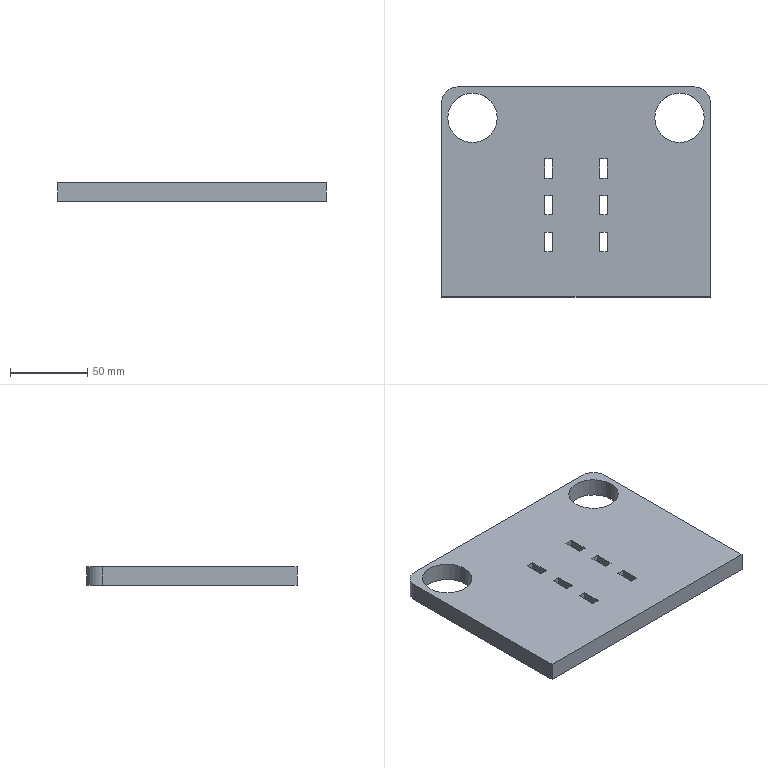Part | SolidWorks | features Extrusion 1, Fillet 1 | 1 solid | 36 faces | box 174 x 136 x 12 mm | volume 259651 mm3 | plane 30 | cylinder 6 | commonest cylinder face diameters 32 x4 20 x2
STEP:
#1=CARTESIAN_POINT('',(28.335,49.66,12.));
#2=VERTEX_POINT('',#1);
#3=CARTESIAN_POINT('',(60.335,49.66,12.));
#4=VERTEX_POINT('',#3);
#5=CARTESIAN_POINT('',(44.335,49.66,12.));
#6=DIRECTION('',(0.,0.,1.));
#7=DIRECTION('',(-1.,0.,0.));
#8=AXIS2_PLACEMENT_3D('',#5,#6,#7);
#9=CIRCLE('',#8,16.);
#10=EDGE_CURVE('',#2,#4,#9,.T.);
#11=ORIENTED_EDGE('',*,*,#10,.T.);
#12=CARTESIAN_POINT('',(60.335,49.66,0.));
#13=VERTEX_POINT('',#12);
#14=CARTESIAN_POINT('',(60.335,49.66,12.));
#15=DIRECTION('',(0.,0.,-1.));
#16=VECTOR('',#15,1000.);
#17=LINE('',#14,#16);
#18=EDGE_CURVE('',#4,#13,#17,.T.);
#19=ORIENTED_EDGE('',*,*,#18,.T.);
#20=CARTESIAN_POINT('',(28.335,49.66,0.));
#21=VERTEX_POINT('',#20);
#22=CARTESIAN_POINT('',(44.335,49.66,0.));
#23=DIRECTION('',(0.,0.,1.));
#24=DIRECTION('',(-1.,0.,0.));
#25=AXIS2_PLACEMENT_3D('',#22,#23,#24);
#26=CIRCLE('',#25,16.);
#27=EDGE_CURVE('',#21,#13,#26,.T.);
#28=ORIENTED_EDGE('',*,*,#27,.F.);
#29=CARTESIAN_POINT('',(28.335,49.66,12.));
#30=DIRECTION('',(0.,0.,-1.));
#31=VECTOR('',#30,1000.);
#32=LINE('',#29,#31);
#33=EDGE_CURVE('',#2,#21,#32,.T.);
#34=ORIENTED_EDGE('',*,*,#33,.F.);
#35=EDGE_LOOP('',(#11,#19,#28,#34));
#36=FACE_OUTER_BOUND('',#35,.T.);
#37=CARTESIAN_POINT('',(44.335,49.66,12.));
#38=DIRECTION('',(0.,0.,-1.));
#39=DIRECTION('',(-1.,0.,0.));
#40=AXIS2_PLACEMENT_3D('',#37,#38,#39);
#41=CYLINDRICAL_SURFACE('',#40,16.);
#42=ADVANCED_FACE('',(#36),#41,.F.);
#43=CARTESIAN_POINT('',(-105.665,49.66,12.));
#44=VERTEX_POINT('',#43);
#45=CARTESIAN_POINT('',(-73.665,49.66,12.));
#46=VERTEX_POINT('',#45);
#47=CARTESIAN_POINT('',(-89.665,49.66,12.));
#48=DIRECTION('',(0.,0.,1.));
#49=DIRECTION('',(1.,0.,0.));
#50=AXIS2_PLACEMENT_3D('',#47,#48,#49);
#51=CIRCLE('',#50,16.);
#52=EDGE_CURVE('',#44,#46,#51,.T.);
#53=ORIENTED_EDGE('',*,*,#52,.T.);
#54=CARTESIAN_POINT('',(-73.665,49.66,0.));
#55=VERTEX_POINT('',#54);
#56=CARTESIAN_POINT('',(-73.665,49.66,12.));
#57=DIRECTION('',(0.,0.,-1.));
#58=VECTOR('',#57,1000.);
#59=LINE('',#56,#58);
#60=EDGE_CURVE('',#46,#55,#59,.T.);
#61=ORIENTED_EDGE('',*,*,#60,.T.);
#62=CARTESIAN_POINT('',(-105.665,49.66,0.));
#63=VERTEX_POINT('',#62);
#64=CARTESIAN_POINT('',(-89.665,49.66,0.));
#65=DIRECTION('',(0.,0.,1.));
#66=DIRECTION('',(1.,0.,0.));
#67=AXIS2_PLACEMENT_3D('',#64,#65,#66);
#68=CIRCLE('',#67,16.);
#69=EDGE_CURVE('',#63,#55,#68,.T.);
#70=ORIENTED_EDGE('',*,*,#69,.F.);
#71=CARTESIAN_POINT('',(-105.665,49.66,12.));
#72=DIRECTION('',(0.,0.,-1.));
#73=VECTOR('',#72,1000.);
#74=LINE('',#71,#73);
#75=EDGE_CURVE('',#44,#63,#74,.T.);
#76=ORIENTED_EDGE('',*,*,#75,.F.);
#77=EDGE_LOOP('',(#53,#61,#70,#76));
#78=FACE_OUTER_BOUND('',#77,.T.);
#79=CARTESIAN_POINT('',(-89.665,49.66,12.));
#80=DIRECTION('',(0.,0.,-1.));
#81=DIRECTION('',(-1.,0.,0.));
#82=AXIS2_PLACEMENT_3D('',#79,#80,#81);
#83=CYLINDRICAL_SURFACE('',#82,16.);
#84=ADVANCED_FACE('',(#78),#83,.F.);
#85=CARTESIAN_POINT('',(-7.415,-0.6475,12.));
#86=VERTEX_POINT('',#85);
#87=CARTESIAN_POINT('',(-7.415,-13.148,12.));
#88=VERTEX_POINT('',#87);
#89=CARTESIAN_POINT('',(-7.415,-0.6475,12.));
#90=DIRECTION('',(0.,-1.,0.));
#91=VECTOR('',#90,1000.);
#92=LINE('',#89,#91);
#93=EDGE_CURVE('',#86,#88,#92,.T.);
#94=ORIENTED_EDGE('',*,*,#93,.F.);
#95=CARTESIAN_POINT('',(-2.415,-0.6475,12.));
#96=VERTEX_POINT('',#95);
#97=CARTESIAN_POINT('',(-7.415,-0.6475,12.));
#98=DIRECTION('',(-1.,0.,0.));
#99=VECTOR('',#98,1000.);
#100=LINE('',#97,#99);
#101=EDGE_CURVE('',#96,#86,#100,.T.);
#102=ORIENTED_EDGE('',*,*,#101,.F.);
#103=CARTESIAN_POINT('',(-2.415,-13.148,12.));
#104=VERTEX_POINT('',#103);
#105=CARTESIAN_POINT('',(-2.415,-0.6475,12.));
#106=DIRECTION('',(0.,1.,0.));
#107=VECTOR('',#106,1000.);
#108=LINE('',#105,#107);
#109=EDGE_CURVE('',#104,#96,#108,.T.);
#110=ORIENTED_EDGE('',*,*,#109,.F.);
#111=CARTESIAN_POINT('',(-2.415,-13.148,12.));
#112=DIRECTION('',(1.,0.,0.));
#113=VECTOR('',#112,1000.);
#114=LINE('',#111,#113);
#115=EDGE_CURVE('',#88,#104,#114,.T.);
#116=ORIENTED_EDGE('',*,*,#115,.F.);
#117=EDGE_LOOP('',(#94,#102,#110,#116));
#118=FACE_BOUND('',#117,.T.);
#119=CARTESIAN_POINT('',(-37.915,-36.898,12.));
#120=VERTEX_POINT('',#119);
#121=CARTESIAN_POINT('',(-37.915,-24.398,12.));
#122=VERTEX_POINT('',#121);
#123=CARTESIAN_POINT('',(-37.915,-24.398,12.));
#124=DIRECTION('',(0.,1.,0.));
#125=VECTOR('',#124,1000.);
#126=LINE('',#123,#125);
#127=EDGE_CURVE('',#120,#122,#126,.T.);
#128=ORIENTED_EDGE('',*,*,#127,.F.);
#129=CARTESIAN_POINT('',(-42.915,-36.898,12.));
#130=VERTEX_POINT('',#129);
#131=CARTESIAN_POINT('',(-42.915,-36.898,12.));
#132=DIRECTION('',(1.,0.,0.));
#133=VECTOR('',#132,1000.);
#134=LINE('',#131,#133);
#135=EDGE_CURVE('',#130,#120,#134,.T.);
#136=ORIENTED_EDGE('',*,*,#135,.F.);
#137=CARTESIAN_POINT('',(-42.915,-24.398,12.));
#138=VERTEX_POINT('',#137);
#139=CARTESIAN_POINT('',(-42.915,-24.398,12.));
#140=DIRECTION('',(0.,-1.,0.));
#141=VECTOR('',#140,1000.);
#142=LINE('',#139,#141);
#143=EDGE_CURVE('',#138,#130,#142,.T.);
#144=ORIENTED_EDGE('',*,*,#143,.F.);
#145=CARTESIAN_POINT('',(-37.915,-24.398,12.));
#146=DIRECTION('',(-1.,0.,0.));
#147=VECTOR('',#146,1000.);
#148=LINE('',#145,#147);
#149=EDGE_CURVE('',#122,#138,#148,.T.);
#150=ORIENTED_EDGE('',*,*,#149,.F.);
#151=EDGE_LOOP('',(#128,#136,#144,#150));
#152=FACE_BOUND('',#151,.T.);
#153=CARTESIAN_POINT('',(-37.915,10.602,12.));
#154=VERTEX_POINT('',#153);
#155=CARTESIAN_POINT('',(-37.915,23.102,12.));
#156=VERTEX_POINT('',#155);
#157=CARTESIAN_POINT('',(-37.915,23.102,12.));
#158=DIRECTION('',(0.,1.,0.));
#159=VECTOR('',#158,1000.);
#160=LINE('',#157,#159);
#161=EDGE_CURVE('',#154,#156,#160,.T.);
#162=ORIENTED_EDGE('',*,*,#161,.F.);
#163=CARTESIAN_POINT('',(-42.915,10.602,12.));
#164=VERTEX_POINT('',#163);
#165=CARTESIAN_POINT('',(-42.915,10.602,12.));
#166=DIRECTION('',(1.,0.,0.));
#167=VECTOR('',#166,1000.);
#168=LINE('',#165,#167);
#169=EDGE_CURVE('',#164,#154,#168,.T.);
#170=ORIENTED_EDGE('',*,*,#169,.F.);
#171=CARTESIAN_POINT('',(-42.915,23.102,12.));
#172=VERTEX_POINT('',#171);
#173=CARTESIAN_POINT('',(-42.915,23.102,12.));
#174=DIRECTION('',(0.,-1.,0.));
#175=VECTOR('',#174,1000.);
#176=LINE('',#173,#175);
#177=EDGE_CURVE('',#172,#164,#176,.T.);
#178=ORIENTED_EDGE('',*,*,#177,.F.);
#179=CARTESIAN_POINT('',(-37.915,23.102,12.));
#180=DIRECTION('',(-1.,0.,0.));
#181=VECTOR('',#180,1000.);
#182=LINE('',#179,#181);
#183=EDGE_CURVE('',#156,#172,#182,.T.);
#184=ORIENTED_EDGE('',*,*,#183,.F.);
#185=EDGE_LOOP('',(#162,#170,#178,#184));
#186=FACE_BOUND('',#185,.T.);
#187=CARTESIAN_POINT('',(64.335,-66.34,12.));
#188=VERTEX_POINT('',#187);
#189=CARTESIAN_POINT('',(64.335,59.66,12.));
#190=VERTEX_POINT('',#189);
#191=CARTESIAN_POINT('',(64.335,69.66,12.));
#192=DIRECTION('',(0.,1.,0.));
#193=VECTOR('',#192,1000.);
#194=LINE('',#191,#193);
#195=EDGE_CURVE('',#188,#190,#194,.T.);
#196=ORIENTED_EDGE('',*,*,#195,.T.);
#197=CARTESIAN_POINT('',(54.335,69.66,12.));
#198=VERTEX_POINT('',#197);
#199=CARTESIAN_POINT('',(54.335,59.66,12.));
#200=DIRECTION('',(0.,0.,1.));
#201=DIRECTION('',(-1.,0.,0.));
#202=AXIS2_PLACEMENT_3D('',#199,#200,#201);
#203=CIRCLE('',#202,10.);
#204=EDGE_CURVE('',#190,#198,#203,.T.);
#205=ORIENTED_EDGE('',*,*,#204,.T.);
#206=CARTESIAN_POINT('',(-99.665,69.66,12.));
#207=VERTEX_POINT('',#206);
#208=CARTESIAN_POINT('',(-109.665,69.66,12.));
#209=DIRECTION('',(-1.,0.,0.));
#210=VECTOR('',#209,1000.);
#211=LINE('',#208,#210);
#212=EDGE_CURVE('',#198,#207,#211,.T.);
#213=ORIENTED_EDGE('',*,*,#212,.T.);
#214=CARTESIAN_POINT('',(-109.665,59.66,12.));
#215=VERTEX_POINT('',#214);
#216=CARTESIAN_POINT('',(-99.665,59.66,12.));
#217=DIRECTION('',(0.,0.,1.));
#218=DIRECTION('',(-1.,0.,0.));
#219=AXIS2_PLACEMENT_3D('',#216,#217,#218);
#220=CIRCLE('',#219,10.);
#221=EDGE_CURVE('',#207,#215,#220,.T.);
#222=ORIENTED_EDGE('',*,*,#221,.T.);
#223=CARTESIAN_POINT('',(-109.665,-66.34,12.));
#224=VERTEX_POINT('',#223);
#225=CARTESIAN_POINT('',(-109.665,69.66,12.));
#226=DIRECTION('',(0.,-1.,0.));
#227=VECTOR('',#226,1000.);
#228=LINE('',#225,#227);
#229=EDGE_CURVE('',#215,#224,#228,.T.);
#230=ORIENTED_EDGE('',*,*,#229,.T.);
#231=CARTESIAN_POINT('',(-109.665,-66.34,12.));
#232=DIRECTION('',(1.,0.,0.));
#233=VECTOR('',#232,1000.);
#234=LINE('',#231,#233);
#235=EDGE_CURVE('',#224,#188,#234,.T.);
#236=ORIENTED_EDGE('',*,*,#235,.T.);
#237=EDGE_LOOP('',(#196,#205,#213,#222,#230,#236));
#238=FACE_OUTER_BOUND('',#237,.T.);
#239=ORIENTED_EDGE('',*,*,#52,.F.);
#240=CARTESIAN_POINT('',(-89.665,49.66,12.));
#241=DIRECTION('',(0.,0.,1.));
#242=DIRECTION('',(1.,0.,0.));
#243=AXIS2_PLACEMENT_3D('',#240,#241,#242);
#244=CIRCLE('',#243,16.);
#245=EDGE_CURVE('',#46,#44,#244,.T.);
#246=ORIENTED_EDGE('',*,*,#245,.F.);
#247=EDGE_LOOP('',(#239,#246));
#248=FACE_BOUND('',#247,.T.);
#249=ORIENTED_EDGE('',*,*,#10,.F.);
#250=CARTESIAN_POINT('',(44.335,49.66,12.));
#251=DIRECTION('',(0.,0.,1.));
#252=DIRECTION('',(-1.,0.,0.));
#253=AXIS2_PLACEMENT_3D('',#250,#251,#252);
#254=CIRCLE('',#253,16.);
#255=EDGE_CURVE('',#4,#2,#254,.T.);
#256=ORIENTED_EDGE('',*,*,#255,.F.);
#257=EDGE_LOOP('',(#249,#256));
#258=FACE_BOUND('',#257,.T.);
#259=CARTESIAN_POINT('',(-37.915,-13.148,12.));
#260=VERTEX_POINT('',#259);
#261=CARTESIAN_POINT('',(-37.915,-0.6475,12.));
#262=VERTEX_POINT('',#261);
#263=CARTESIAN_POINT('',(-37.915,-0.6475,12.));
#264=DIRECTION('',(0.,1.,0.));
#265=VECTOR('',#264,1000.);
#266=LINE('',#263,#265);
#267=EDGE_CURVE('',#260,#262,#266,.T.);
#268=ORIENTED_EDGE('',*,*,#267,.F.);
#269=CARTESIAN_POINT('',(-42.915,-13.148,12.));
#270=VERTEX_POINT('',#269);
#271=CARTESIAN_POINT('',(-42.915,-13.148,12.));
#272=DIRECTION('',(1.,0.,0.));
#273=VECTOR('',#272,1000.);
#274=LINE('',#271,#273);
#275=EDGE_CURVE('',#270,#260,#274,.T.);
#276=ORIENTED_EDGE('',*,*,#275,.F.);
#277=CARTESIAN_POINT('',(-42.915,-0.6475,12.));
#278=VERTEX_POINT('',#277);
#279=CARTESIAN_POINT('',(-42.915,-0.6475,12.));
#280=DIRECTION('',(0.,-1.,0.));
#281=VECTOR('',#280,1000.);
#282=LINE('',#279,#281);
#283=EDGE_CURVE('',#278,#270,#282,.T.);
#284=ORIENTED_EDGE('',*,*,#283,.F.);
#285=CARTESIAN_POINT('',(-37.915,-0.6475,12.));
#286=DIRECTION('',(-1.,0.,0.));
#287=VECTOR('',#286,1000.);
#288=LINE('',#285,#287);
#289=EDGE_CURVE('',#262,#278,#288,.T.);
#290=ORIENTED_EDGE('',*,*,#289,.F.);
#291=EDGE_LOOP('',(#268,#276,#284,#290));
#292=FACE_BOUND('',#291,.T.);
#293=CARTESIAN_POINT('',(-7.415,-24.398,12.));
#294=VERTEX_POINT('',#293);
#295=CARTESIAN_POINT('',(-7.415,-36.898,12.));
#296=VERTEX_POINT('',#295);
#297=CARTESIAN_POINT('',(-7.415,-24.398,12.));
#298=DIRECTION('',(0.,-1.,0.));
#299=VECTOR('',#298,1000.);
#300=LINE('',#297,#299);
#301=EDGE_CURVE('',#294,#296,#300,.T.);
#302=ORIENTED_EDGE('',*,*,#301,.F.);
#303=CARTESIAN_POINT('',(-2.415,-24.398,12.));
#304=VERTEX_POINT('',#303);
#305=CARTESIAN_POINT('',(-7.415,-24.398,12.));
#306=DIRECTION('',(-1.,0.,0.));
#307=VECTOR('',#306,1000.);
#308=LINE('',#305,#307);
#309=EDGE_CURVE('',#304,#294,#308,.T.);
#310=ORIENTED_EDGE('',*,*,#309,.F.);
#311=CARTESIAN_POINT('',(-2.415,-36.898,12.));
#312=VERTEX_POINT('',#311);
#313=CARTESIAN_POINT('',(-2.415,-24.398,12.));
#314=DIRECTION('',(0.,1.,0.));
#315=VECTOR('',#314,1000.);
#316=LINE('',#313,#315);
#317=EDGE_CURVE('',#312,#304,#316,.T.);
#318=ORIENTED_EDGE('',*,*,#317,.F.);
#319=CARTESIAN_POINT('',(-2.415,-36.898,12.));
#320=DIRECTION('',(1.,0.,0.));
#321=VECTOR('',#320,1000.);
#322=LINE('',#319,#321);
#323=EDGE_CURVE('',#296,#312,#322,.T.);
#324=ORIENTED_EDGE('',*,*,#323,.F.);
#325=EDGE_LOOP('',(#302,#310,#318,#324));
#326=FACE_BOUND('',#325,.T.);
#327=CARTESIAN_POINT('',(-7.415,23.102,12.));
#328=VERTEX_POINT('',#327);
#329=CARTESIAN_POINT('',(-7.415,10.602,12.));
#330=VERTEX_POINT('',#329);
#331=CARTESIAN_POINT('',(-7.415,23.102,12.));
#332=DIRECTION('',(0.,-1.,0.));
#333=VECTOR('',#332,1000.);
#334=LINE('',#331,#333);
#335=EDGE_CURVE('',#328,#330,#334,.T.);
#336=ORIENTED_EDGE('',*,*,#335,.F.);
#337=CARTESIAN_POINT('',(-2.415,23.102,12.));
#338=VERTEX_POINT('',#337);
#339=CARTESIAN_POINT('',(-7.415,23.102,12.));
#340=DIRECTION('',(-1.,0.,0.));
#341=VECTOR('',#340,1000.);
#342=LINE('',#339,#341);
#343=EDGE_CURVE('',#338,#328,#342,.T.);
#344=ORIENTED_EDGE('',*,*,#343,.F.);
#345=CARTESIAN_POINT('',(-2.415,10.602,12.));
#346=VERTEX_POINT('',#345);
#347=CARTESIAN_POINT('',(-2.415,23.102,12.));
#348=DIRECTION('',(0.,1.,0.));
#349=VECTOR('',#348,1000.);
#350=LINE('',#347,#349);
#351=EDGE_CURVE('',#346,#338,#350,.T.);
#352=ORIENTED_EDGE('',*,*,#351,.F.);
#353=CARTESIAN_POINT('',(-2.415,10.602,12.));
#354=DIRECTION('',(1.,0.,0.));
#355=VECTOR('',#354,1000.);
#356=LINE('',#353,#355);
#357=EDGE_CURVE('',#330,#346,#356,.T.);
#358=ORIENTED_EDGE('',*,*,#357,.F.);
#359=EDGE_LOOP('',(#336,#344,#352,#358));
#360=FACE_BOUND('',#359,.T.);
#361=CARTESIAN_POINT('',(0.,0.,12.));
#362=DIRECTION('',(0.,0.,-1.));
#363=DIRECTION('',(-1.,0.,0.));
#364=AXIS2_PLACEMENT_3D('',#361,#362,#363);
#365=PLANE('',#364);
#366=ADVANCED_FACE('',(#118,#152,#186,#238,#248,#258,#292,#326,#360),#365,.F.);
#367=ORIENTED_EDGE('',*,*,#69,.T.);
#368=CARTESIAN_POINT('',(-89.665,49.66,0.));
#369=DIRECTION('',(0.,0.,1.));
#370=DIRECTION('',(1.,0.,0.));
#371=AXIS2_PLACEMENT_3D('',#368,#369,#370);
#372=CIRCLE('',#371,16.);
#373=EDGE_CURVE('',#55,#63,#372,.T.);
#374=ORIENTED_EDGE('',*,*,#373,.T.);
#375=EDGE_LOOP('',(#367,#374));
#376=FACE_BOUND('',#375,.T.);
#377=CARTESIAN_POINT('',(54.335,69.66,0.));
#378=VERTEX_POINT('',#377);
#379=CARTESIAN_POINT('',(-99.665,69.66,0.));
#380=VERTEX_POINT('',#379);
#381=CARTESIAN_POINT('',(-109.665,69.66,0.));
#382=DIRECTION('',(-1.,0.,0.));
#383=VECTOR('',#382,1000.);
#384=LINE('',#381,#383);
#385=EDGE_CURVE('',#378,#380,#384,.T.);
#386=ORIENTED_EDGE('',*,*,#385,.F.);
#387=CARTESIAN_POINT('',(64.335,59.66,0.));
#388=VERTEX_POINT('',#387);
#389=CARTESIAN_POINT('',(54.335,59.66,0.));
#390=DIRECTION('',(0.,0.,-1.));
#391=DIRECTION('',(-1.,0.,0.));
#392=AXIS2_PLACEMENT_3D('',#389,#390,#391);
#393=CIRCLE('',#392,10.);
#394=EDGE_CURVE('',#378,#388,#393,.T.);
#395=ORIENTED_EDGE('',*,*,#394,.T.);
#396=CARTESIAN_POINT('',(64.335,-66.34,0.));
#397=VERTEX_POINT('',#396);
#398=CARTESIAN_POINT('',(64.335,69.66,0.));
#399=DIRECTION('',(0.,1.,0.));
#400=VECTOR('',#399,1000.);
#401=LINE('',#398,#400);
#402=EDGE_CURVE('',#397,#388,#401,.T.);
#403=ORIENTED_EDGE('',*,*,#402,.F.);
#404=CARTESIAN_POINT('',(-109.665,-66.34,0.));
#405=VERTEX_POINT('',#404);
#406=CARTESIAN_POINT('',(-109.665,-66.34,0.));
#407=DIRECTION('',(1.,0.,0.));
#408=VECTOR('',#407,1000.);
#409=LINE('',#406,#408);
#410=EDGE_CURVE('',#405,#397,#409,.T.);
#411=ORIENTED_EDGE('',*,*,#410,.F.);
#412=CARTESIAN_POINT('',(-109.665,59.66,0.));
#413=VERTEX_POINT('',#412);
#414=CARTESIAN_POINT('',(-109.665,69.66,0.));
#415=DIRECTION('',(0.,-1.,0.));
#416=VECTOR('',#415,1000.);
#417=LINE('',#414,#416);
#418=EDGE_CURVE('',#413,#405,#417,.T.);
#419=ORIENTED_EDGE('',*,*,#418,.F.);
#420=CARTESIAN_POINT('',(-99.665,59.66,0.));
#421=DIRECTION('',(0.,0.,-1.));
#422=DIRECTION('',(-1.,0.,0.));
#423=AXIS2_PLACEMENT_3D('',#420,#421,#422);
#424=CIRCLE('',#423,10.);
#425=EDGE_CURVE('',#413,#380,#424,.T.);
#426=ORIENTED_EDGE('',*,*,#425,.T.);
#427=EDGE_LOOP('',(#386,#395,#403,#411,#419,#426));
#428=FACE_OUTER_BOUND('',#427,.T.);
#429=ORIENTED_EDGE('',*,*,#27,.T.);
#430=CARTESIAN_POINT('',(44.335,49.66,0.));
#431=DIRECTION('',(0.,0.,1.));
#432=DIRECTION('',(-1.,0.,0.));
#433=AXIS2_PLACEMENT_3D('',#430,#431,#432);
#434=CIRCLE('',#433,16.);
#435=EDGE_CURVE('',#13,#21,#434,.T.);
#436=ORIENTED_EDGE('',*,*,#435,.T.);
#437=EDGE_LOOP('',(#429,#436));
#438=FACE_BOUND('',#437,.T.);
#439=CARTESIAN_POINT('',(-42.915,10.602,0.));
#440=VERTEX_POINT('',#439);
#441=CARTESIAN_POINT('',(-37.915,10.602,0.));
#442=VERTEX_POINT('',#441);
#443=CARTESIAN_POINT('',(-42.915,10.602,0.));
#444=DIRECTION('',(1.,0.,0.));
#445=VECTOR('',#444,1000.);
#446=LINE('',#443,#445);
#447=EDGE_CURVE('',#440,#442,#446,.T.);
#448=ORIENTED_EDGE('',*,*,#447,.T.);
#449=CARTESIAN_POINT('',(-37.915,23.102,0.));
#450=VERTEX_POINT('',#449);
#451=CARTESIAN_POINT('',(-37.915,23.102,0.));
#452=DIRECTION('',(0.,1.,0.));
#453=VECTOR('',#452,1000.);
#454=LINE('',#451,#453);
#455=EDGE_CURVE('',#442,#450,#454,.T.);
#456=ORIENTED_EDGE('',*,*,#455,.T.);
#457=CARTESIAN_POINT('',(-42.915,23.102,0.));
#458=VERTEX_POINT('',#457);
#459=CARTESIAN_POINT('',(-37.915,23.102,0.));
#460=DIRECTION('',(-1.,0.,0.));
#461=VECTOR('',#460,1000.);
#462=LINE('',#459,#461);
#463=EDGE_CURVE('',#450,#458,#462,.T.);
#464=ORIENTED_EDGE('',*,*,#463,.T.);
#465=CARTESIAN_POINT('',(-42.915,23.102,0.));
#466=DIRECTION('',(0.,-1.,0.));
#467=VECTOR('',#466,1000.);
#468=LINE('',#465,#467);
#469=EDGE_CURVE('',#458,#440,#468,.T.);
#470=ORIENTED_EDGE('',*,*,#469,.T.);
#471=EDGE_LOOP('',(#448,#456,#464,#470));
#472=FACE_BOUND('',#471,.T.);
#473=CARTESIAN_POINT('',(-42.915,-13.148,0.));
#474=VERTEX_POINT('',#473);
#475=CARTESIAN_POINT('',(-37.915,-13.148,0.));
#476=VERTEX_POINT('',#475);
#477=CARTESIAN_POINT('',(-42.915,-13.148,0.));
#478=DIRECTION('',(1.,0.,0.));
#479=VECTOR('',#478,1000.);
#480=LINE('',#477,#479);
#481=EDGE_CURVE('',#474,#476,#480,.T.);
#482=ORIENTED_EDGE('',*,*,#481,.T.);
#483=CARTESIAN_POINT('',(-37.915,-0.6475,0.));
#484=VERTEX_POINT('',#483);
#485=CARTESIAN_POINT('',(-37.915,-0.6475,0.));
#486=DIRECTION('',(0.,1.,0.));
#487=VECTOR('',#486,1000.);
#488=LINE('',#485,#487);
#489=EDGE_CURVE('',#476,#484,#488,.T.);
#490=ORIENTED_EDGE('',*,*,#489,.T.);
#491=CARTESIAN_POINT('',(-42.915,-0.6475,0.));
#492=VERTEX_POINT('',#491);
#493=CARTESIAN_POINT('',(-37.915,-0.6475,0.));
#494=DIRECTION('',(-1.,0.,0.));
#495=VECTOR('',#494,1000.);
#496=LINE('',#493,#495);
#497=EDGE_CURVE('',#484,#492,#496,.T.);
#498=ORIENTED_EDGE('',*,*,#497,.T.);
#499=CARTESIAN_POINT('',(-42.915,-0.6475,0.));
#500=DIRECTION('',(0.,-1.,0.));
#501=VECTOR('',#500,1000.);
#502=LINE('',#499,#501);
#503=EDGE_CURVE('',#492,#474,#502,.T.);
#504=ORIENTED_EDGE('',*,*,#503,.T.);
#505=EDGE_LOOP('',(#482,#490,#498,#504));
#506=FACE_BOUND('',#505,.T.);
#507=CARTESIAN_POINT('',(-42.915,-36.898,0.));
#508=VERTEX_POINT('',#507);
#509=CARTESIAN_POINT('',(-37.915,-36.898,0.));
#510=VERTEX_POINT('',#509);
#511=CARTESIAN_POINT('',(-42.915,-36.898,0.));
#512=DIRECTION('',(1.,0.,0.));
#513=VECTOR('',#512,1000.);
#514=LINE('',#511,#513);
#515=EDGE_CURVE('',#508,#510,#514,.T.);
#516=ORIENTED_EDGE('',*,*,#515,.T.);
#517=CARTESIAN_POINT('',(-37.915,-24.398,0.));
#518=VERTEX_POINT('',#517);
#519=CARTESIAN_POINT('',(-37.915,-24.398,0.));
#520=DIRECTION('',(0.,1.,0.));
#521=VECTOR('',#520,1000.);
#522=LINE('',#519,#521);
#523=EDGE_CURVE('',#510,#518,#522,.T.);
#524=ORIENTED_EDGE('',*,*,#523,.T.);
#525=CARTESIAN_POINT('',(-42.915,-24.398,0.));
#526=VERTEX_POINT('',#525);
#527=CARTESIAN_POINT('',(-37.915,-24.398,0.));
#528=DIRECTION('',(-1.,0.,0.));
#529=VECTOR('',#528,1000.);
#530=LINE('',#527,#529);
#531=EDGE_CURVE('',#518,#526,#530,.T.);
#532=ORIENTED_EDGE('',*,*,#531,.T.);
#533=CARTESIAN_POINT('',(-42.915,-24.398,0.));
#534=DIRECTION('',(0.,-1.,0.));
#535=VECTOR('',#534,1000.);
#536=LINE('',#533,#535);
#537=EDGE_CURVE('',#526,#508,#536,.T.);
#538=ORIENTED_EDGE('',*,*,#537,.T.);
#539=EDGE_LOOP('',(#516,#524,#532,#538));
#540=FACE_BOUND('',#539,.T.);
#541=CARTESIAN_POINT('',(-2.415,-24.398,0.));
#542=VERTEX_POINT('',#541);
#543=CARTESIAN_POINT('',(-7.415,-24.398,0.));
#544=VERTEX_POINT('',#543);
#545=CARTESIAN_POINT('',(-7.415,-24.398,0.));
#546=DIRECTION('',(-1.,0.,0.));
#547=VECTOR('',#546,1000.);
#548=LINE('',#545,#547);
#549=EDGE_CURVE('',#542,#544,#548,.T.);
#550=ORIENTED_EDGE('',*,*,#549,.T.);
#551=CARTESIAN_POINT('',(-7.415,-36.898,0.));
#552=VERTEX_POINT('',#551);
#553=CARTESIAN_POINT('',(-7.415,-24.398,0.));
#554=DIRECTION('',(0.,-1.,0.));
#555=VECTOR('',#554,1000.);
#556=LINE('',#553,#555);
#557=EDGE_CURVE('',#544,#552,#556,.T.);
#558=ORIENTED_EDGE('',*,*,#557,.T.);
#559=CARTESIAN_POINT('',(-2.415,-36.898,0.));
#560=VERTEX_POINT('',#559);
#561=CARTESIAN_POINT('',(-2.415,-36.898,0.));
#562=DIRECTION('',(1.,0.,0.));
#563=VECTOR('',#562,1000.);
#564=LINE('',#561,#563);
#565=EDGE_CURVE('',#552,#560,#564,.T.);
#566=ORIENTED_EDGE('',*,*,#565,.T.);
#567=CARTESIAN_POINT('',(-2.415,-24.398,0.));
#568=DIRECTION('',(0.,1.,0.));
#569=VECTOR('',#568,1000.);
#570=LINE('',#567,#569);
#571=EDGE_CURVE('',#560,#542,#570,.T.);
#572=ORIENTED_EDGE('',*,*,#571,.T.);
#573=EDGE_LOOP('',(#550,#558,#566,#572));
#574=FACE_BOUND('',#573,.T.);
#575=CARTESIAN_POINT('',(-2.415,-0.6475,0.));
#576=VERTEX_POINT('',#575);
#577=CARTESIAN_POINT('',(-7.415,-0.6475,0.));
#578=VERTEX_POINT('',#577);
#579=CARTESIAN_POINT('',(-7.415,-0.6475,0.));
#580=DIRECTION('',(-1.,0.,0.));
#581=VECTOR('',#580,1000.);
#582=LINE('',#579,#581);
#583=EDGE_CURVE('',#576,#578,#582,.T.);
#584=ORIENTED_EDGE('',*,*,#583,.T.);
#585=CARTESIAN_POINT('',(-7.415,-13.148,0.));
#586=VERTEX_POINT('',#585);
#587=CARTESIAN_POINT('',(-7.415,-0.6475,0.));
#588=DIRECTION('',(0.,-1.,0.));
#589=VECTOR('',#588,1000.);
#590=LINE('',#587,#589);
#591=EDGE_CURVE('',#578,#586,#590,.T.);
#592=ORIENTED_EDGE('',*,*,#591,.T.);
#593=CARTESIAN_POINT('',(-2.415,-13.148,0.));
#594=VERTEX_POINT('',#593);
#595=CARTESIAN_POINT('',(-2.415,-13.148,0.));
#596=DIRECTION('',(1.,0.,0.));
#597=VECTOR('',#596,1000.);
#598=LINE('',#595,#597);
#599=EDGE_CURVE('',#586,#594,#598,.T.);
#600=ORIENTED_EDGE('',*,*,#599,.T.);
#601=CARTESIAN_POINT('',(-2.415,-0.6475,0.));
#602=DIRECTION('',(0.,1.,0.));
#603=VECTOR('',#602,1000.);
#604=LINE('',#601,#603);
#605=EDGE_CURVE('',#594,#576,#604,.T.);
#606=ORIENTED_EDGE('',*,*,#605,.T.);
#607=EDGE_LOOP('',(#584,#592,#600,#606));
#608=FACE_BOUND('',#607,.T.);
#609=CARTESIAN_POINT('',(-2.415,23.102,0.));
#610=VERTEX_POINT('',#609);
#611=CARTESIAN_POINT('',(-7.415,23.102,0.));
#612=VERTEX_POINT('',#611);
#613=CARTESIAN_POINT('',(-7.415,23.102,0.));
#614=DIRECTION('',(-1.,0.,0.));
#615=VECTOR('',#614,1000.);
#616=LINE('',#613,#615);
#617=EDGE_CURVE('',#610,#612,#616,.T.);
#618=ORIENTED_EDGE('',*,*,#617,.T.);
#619=CARTESIAN_POINT('',(-7.415,10.602,0.));
#620=VERTEX_POINT('',#619);
#621=CARTESIAN_POINT('',(-7.415,23.102,0.));
#622=DIRECTION('',(0.,-1.,0.));
#623=VECTOR('',#622,1000.);
#624=LINE('',#621,#623);
#625=EDGE_CURVE('',#612,#620,#624,.T.);
#626=ORIENTED_EDGE('',*,*,#625,.T.);
#627=CARTESIAN_POINT('',(-2.415,10.602,0.));
#628=VERTEX_POINT('',#627);
#629=CARTESIAN_POINT('',(-2.415,10.602,0.));
#630=DIRECTION('',(1.,0.,0.));
#631=VECTOR('',#630,1000.);
#632=LINE('',#629,#631);
#633=EDGE_CURVE('',#620,#628,#632,.T.);
#634=ORIENTED_EDGE('',*,*,#633,.T.);
#635=CARTESIAN_POINT('',(-2.415,23.102,0.));
#636=DIRECTION('',(0.,1.,0.));
#637=VECTOR('',#636,1000.);
#638=LINE('',#635,#637);
#639=EDGE_CURVE('',#628,#610,#638,.T.);
#640=ORIENTED_EDGE('',*,*,#639,.T.);
#641=EDGE_LOOP('',(#618,#626,#634,#640));
#642=FACE_BOUND('',#641,.T.);
#643=CARTESIAN_POINT('',(0.,0.,0.));
#644=DIRECTION('',(0.,0.,-1.));
#645=DIRECTION('',(-1.,0.,0.));
#646=AXIS2_PLACEMENT_3D('',#643,#644,#645);
#647=PLANE('',#646);
#648=ADVANCED_FACE('',(#376,#428,#438,#472,#506,#540,#574,#608,#642),#647,.T.);
#649=ORIENTED_EDGE('',*,*,#212,.F.);
#650=CARTESIAN_POINT('',(54.335,69.66,12.));
#651=DIRECTION('',(0.,0.,-1.));
#652=VECTOR('',#651,1000.);
#653=LINE('',#650,#652);
#654=EDGE_CURVE('',#198,#378,#653,.T.);
#655=ORIENTED_EDGE('',*,*,#654,.T.);
#656=ORIENTED_EDGE('',*,*,#385,.T.);
#657=CARTESIAN_POINT('',(-99.665,69.66,12.));
#658=DIRECTION('',(0.,0.,1.));
#659=VECTOR('',#658,1000.);
#660=LINE('',#657,#659);
#661=EDGE_CURVE('',#380,#207,#660,.T.);
#662=ORIENTED_EDGE('',*,*,#661,.T.);
#663=EDGE_LOOP('',(#649,#655,#656,#662));
#664=FACE_OUTER_BOUND('',#663,.T.);
#665=CARTESIAN_POINT('',(-109.665,69.66,12.));
#666=DIRECTION('',(0.,-1.,0.));
#667=DIRECTION('',(0.,0.,-1.));
#668=AXIS2_PLACEMENT_3D('',#665,#666,#667);
#669=PLANE('',#668);
#670=ADVANCED_FACE('',(#664),#669,.F.);
#671=ORIENTED_EDGE('',*,*,#229,.F.);
#672=CARTESIAN_POINT('',(-109.665,59.66,12.));
#673=DIRECTION('',(0.,0.,-1.));
#674=VECTOR('',#673,1000.);
#675=LINE('',#672,#674);
#676=EDGE_CURVE('',#215,#413,#675,.T.);
#677=ORIENTED_EDGE('',*,*,#676,.T.);
#678=ORIENTED_EDGE('',*,*,#418,.T.);
#679=CARTESIAN_POINT('',(-109.665,-66.34,12.));
#680=DIRECTION('',(0.,0.,-1.));
#681=VECTOR('',#680,1000.);
#682=LINE('',#679,#681);
#683=EDGE_CURVE('',#224,#405,#682,.T.);
#684=ORIENTED_EDGE('',*,*,#683,.F.);
#685=EDGE_LOOP('',(#671,#677,#678,#684));
#686=FACE_OUTER_BOUND('',#685,.T.);
#687=CARTESIAN_POINT('',(-109.665,69.66,12.));
#688=DIRECTION('',(1.,0.,0.));
#689=DIRECTION('',(0.,1.,0.));
#690=AXIS2_PLACEMENT_3D('',#687,#688,#689);
#691=PLANE('',#690);
#692=ADVANCED_FACE('',(#686),#691,.F.);
#693=ORIENTED_EDGE('',*,*,#410,.T.);
#694=CARTESIAN_POINT('',(64.335,-66.34,12.));
#695=DIRECTION('',(0.,0.,-1.));
#696=VECTOR('',#695,1000.);
#697=LINE('',#694,#696);
#698=EDGE_CURVE('',#188,#397,#697,.T.);
#699=ORIENTED_EDGE('',*,*,#698,.F.);
#700=ORIENTED_EDGE('',*,*,#235,.F.);
#701=ORIENTED_EDGE('',*,*,#683,.T.);
#702=EDGE_LOOP('',(#693,#699,#700,#701));
#703=FACE_OUTER_BOUND('',#702,.T.);
#704=CARTESIAN_POINT('',(-109.665,-66.34,12.));
#705=DIRECTION('',(0.,1.,0.));
#706=DIRECTION('',(0.,0.,1.));
#707=AXIS2_PLACEMENT_3D('',#704,#705,#706);
#708=PLANE('',#707);
#709=ADVANCED_FACE('',(#703),#708,.F.);
#710=ORIENTED_EDGE('',*,*,#402,.T.);
#711=CARTESIAN_POINT('',(64.335,59.66,12.));
#712=DIRECTION('',(0.,0.,1.));
#713=VECTOR('',#712,1000.);
#714=LINE('',#711,#713);
#715=EDGE_CURVE('',#388,#190,#714,.T.);
#716=ORIENTED_EDGE('',*,*,#715,.T.);
#717=ORIENTED_EDGE('',*,*,#195,.F.);
#718=ORIENTED_EDGE('',*,*,#698,.T.);
#719=EDGE_LOOP('',(#710,#716,#717,#718));
#720=FACE_OUTER_BOUND('',#719,.T.);
#721=CARTESIAN_POINT('',(64.335,69.66,12.));
#722=DIRECTION('',(-1.,0.,0.));
#723=DIRECTION('',(0.,-1.,0.));
#724=AXIS2_PLACEMENT_3D('',#721,#722,#723);
#725=PLANE('',#724);
#726=ADVANCED_FACE('',(#720),#725,.F.);
#727=ORIENTED_EDGE('',*,*,#60,.F.);
#728=ORIENTED_EDGE('',*,*,#245,.T.);
#729=ORIENTED_EDGE('',*,*,#75,.T.);
#730=ORIENTED_EDGE('',*,*,#373,.F.);
#731=EDGE_LOOP('',(#727,#728,#729,#730));
#732=FACE_OUTER_BOUND('',#731,.T.);
#733=CARTESIAN_POINT('',(-89.665,49.66,12.));
#734=DIRECTION('',(0.,0.,-1.));
#735=DIRECTION('',(-1.,0.,0.));
#736=AXIS2_PLACEMENT_3D('',#733,#734,#735);
#737=CYLINDRICAL_SURFACE('',#736,16.);
#738=ADVANCED_FACE('',(#732),#737,.F.);
#739=ORIENTED_EDGE('',*,*,#18,.F.);
#740=ORIENTED_EDGE('',*,*,#255,.T.);
#741=ORIENTED_EDGE('',*,*,#33,.T.);
#742=ORIENTED_EDGE('',*,*,#435,.F.);
#743=EDGE_LOOP('',(#739,#740,#741,#742));
#744=FACE_OUTER_BOUND('',#743,.T.);
#745=CARTESIAN_POINT('',(44.335,49.66,12.));
#746=DIRECTION('',(0.,0.,-1.));
#747=DIRECTION('',(-1.,0.,0.));
#748=AXIS2_PLACEMENT_3D('',#745,#746,#747);
#749=CYLINDRICAL_SURFACE('',#748,16.);
#750=ADVANCED_FACE('',(#744),#749,.F.);
#751=ORIENTED_EDGE('',*,*,#455,.F.);
#752=CARTESIAN_POINT('',(-37.915,10.602,12.));
#753=DIRECTION('',(0.,0.,-1.));
#754=VECTOR('',#753,1000.);
#755=LINE('',#752,#754);
#756=EDGE_CURVE('',#154,#442,#755,.T.);
#757=ORIENTED_EDGE('',*,*,#756,.F.);
#758=ORIENTED_EDGE('',*,*,#161,.T.);
#759=CARTESIAN_POINT('',(-37.915,23.102,12.));
#760=DIRECTION('',(0.,0.,-1.));
#761=VECTOR('',#760,1000.);
#762=LINE('',#759,#761);
#763=EDGE_CURVE('',#156,#450,#762,.T.);
#764=ORIENTED_EDGE('',*,*,#763,.T.);
#765=EDGE_LOOP('',(#751,#757,#758,#764));
#766=FACE_OUTER_BOUND('',#765,.T.);
#767=CARTESIAN_POINT('',(-37.915,23.102,12.));
#768=DIRECTION('',(-1.,0.,0.));
#769=DIRECTION('',(0.,0.,1.));
#770=AXIS2_PLACEMENT_3D('',#767,#768,#769);
#771=PLANE('',#770);
#772=ADVANCED_FACE('',(#766),#771,.T.);
#773=ORIENTED_EDGE('',*,*,#463,.F.);
#774=ORIENTED_EDGE('',*,*,#763,.F.);
#775=ORIENTED_EDGE('',*,*,#183,.T.);
#776=CARTESIAN_POINT('',(-42.915,23.102,12.));
#777=DIRECTION('',(0.,0.,-1.));
#778=VECTOR('',#777,1000.);
#779=LINE('',#776,#778);
#780=EDGE_CURVE('',#172,#458,#779,.T.);
#781=ORIENTED_EDGE('',*,*,#780,.T.);
#782=EDGE_LOOP('',(#773,#774,#775,#781));
#783=FACE_OUTER_BOUND('',#782,.T.);
#784=CARTESIAN_POINT('',(-37.915,23.102,12.));
#785=DIRECTION('',(0.,-1.,0.));
#786=DIRECTION('',(0.,0.,-1.));
#787=AXIS2_PLACEMENT_3D('',#784,#785,#786);
#788=PLANE('',#787);
#789=ADVANCED_FACE('',(#783),#788,.T.);
#790=ORIENTED_EDGE('',*,*,#469,.F.);
#791=ORIENTED_EDGE('',*,*,#780,.F.);
#792=ORIENTED_EDGE('',*,*,#177,.T.);
#793=CARTESIAN_POINT('',(-42.915,10.602,12.));
#794=DIRECTION('',(0.,0.,-1.));
#795=VECTOR('',#794,1000.);
#796=LINE('',#793,#795);
#797=EDGE_CURVE('',#164,#440,#796,.T.);
#798=ORIENTED_EDGE('',*,*,#797,.T.);
#799=EDGE_LOOP('',(#790,#791,#792,#798));
#800=FACE_OUTER_BOUND('',#799,.T.);
#801=CARTESIAN_POINT('',(-42.915,23.102,12.));
#802=DIRECTION('',(1.,0.,0.));
#803=DIRECTION('',(0.,0.,-1.));
#804=AXIS2_PLACEMENT_3D('',#801,#802,#803);
#805=PLANE('',#804);
#806=ADVANCED_FACE('',(#800),#805,.T.);
#807=ORIENTED_EDGE('',*,*,#447,.F.);
#808=ORIENTED_EDGE('',*,*,#797,.F.);
#809=ORIENTED_EDGE('',*,*,#169,.T.);
#810=ORIENTED_EDGE('',*,*,#756,.T.);
#811=EDGE_LOOP('',(#807,#808,#809,#810));
#812=FACE_OUTER_BOUND('',#811,.T.);
#813=CARTESIAN_POINT('',(-42.915,10.602,12.));
#814=DIRECTION('',(0.,1.,0.));
#815=DIRECTION('',(-1.,0.,0.));
#816=AXIS2_PLACEMENT_3D('',#813,#814,#815);
#817=PLANE('',#816);
#818=ADVANCED_FACE('',(#812),#817,.T.);
#819=ORIENTED_EDGE('',*,*,#489,.F.);
#820=CARTESIAN_POINT('',(-37.915,-13.148,12.));
#821=DIRECTION('',(0.,0.,-1.));
#822=VECTOR('',#821,1000.);
#823=LINE('',#820,#822);
#824=EDGE_CURVE('',#260,#476,#823,.T.);
#825=ORIENTED_EDGE('',*,*,#824,.F.);
#826=ORIENTED_EDGE('',*,*,#267,.T.);
#827=CARTESIAN_POINT('',(-37.915,-0.6475,12.));
#828=DIRECTION('',(0.,0.,-1.));
#829=VECTOR('',#828,1000.);
#830=LINE('',#827,#829);
#831=EDGE_CURVE('',#262,#484,#830,.T.);
#832=ORIENTED_EDGE('',*,*,#831,.T.);
#833=EDGE_LOOP('',(#819,#825,#826,#832));
#834=FACE_OUTER_BOUND('',#833,.T.);
#835=CARTESIAN_POINT('',(-37.915,-0.6475,12.));
#836=DIRECTION('',(-1.,0.,0.));
#837=DIRECTION('',(0.,-1.,0.));
#838=AXIS2_PLACEMENT_3D('',#835,#836,#837);
#839=PLANE('',#838);
#840=ADVANCED_FACE('',(#834),#839,.T.);
#841=ORIENTED_EDGE('',*,*,#497,.F.);
#842=ORIENTED_EDGE('',*,*,#831,.F.);
#843=ORIENTED_EDGE('',*,*,#289,.T.);
#844=CARTESIAN_POINT('',(-42.915,-0.6475,12.));
#845=DIRECTION('',(0.,0.,-1.));
#846=VECTOR('',#845,1000.);
#847=LINE('',#844,#846);
#848=EDGE_CURVE('',#278,#492,#847,.T.);
#849=ORIENTED_EDGE('',*,*,#848,.T.);
#850=EDGE_LOOP('',(#841,#842,#843,#849));
#851=FACE_OUTER_BOUND('',#850,.T.);
#852=CARTESIAN_POINT('',(-37.915,-0.6475,12.));
#853=DIRECTION('',(0.,-1.,0.));
#854=DIRECTION('',(1.,0.,0.));
#855=AXIS2_PLACEMENT_3D('',#852,#853,#854);
#856=PLANE('',#855);
#857=ADVANCED_FACE('',(#851),#856,.T.);
#858=ORIENTED_EDGE('',*,*,#503,.F.);
#859=ORIENTED_EDGE('',*,*,#848,.F.);
#860=ORIENTED_EDGE('',*,*,#283,.T.);
#861=CARTESIAN_POINT('',(-42.915,-13.148,12.));
#862=DIRECTION('',(0.,0.,-1.));
#863=VECTOR('',#862,1000.);
#864=LINE('',#861,#863);
#865=EDGE_CURVE('',#270,#474,#864,.T.);
#866=ORIENTED_EDGE('',*,*,#865,.T.);
#867=EDGE_LOOP('',(#858,#859,#860,#866));
#868=FACE_OUTER_BOUND('',#867,.T.);
#869=CARTESIAN_POINT('',(-42.915,-0.6475,12.));
#870=DIRECTION('',(1.,0.,0.));
#871=DIRECTION('',(0.,1.,0.));
#872=AXIS2_PLACEMENT_3D('',#869,#870,#871);
#873=PLANE('',#872);
#874=ADVANCED_FACE('',(#868),#873,.T.);
#875=ORIENTED_EDGE('',*,*,#481,.F.);
#876=ORIENTED_EDGE('',*,*,#865,.F.);
#877=ORIENTED_EDGE('',*,*,#275,.T.);
#878=ORIENTED_EDGE('',*,*,#824,.T.);
#879=EDGE_LOOP('',(#875,#876,#877,#878));
#880=FACE_OUTER_BOUND('',#879,.T.);
#881=CARTESIAN_POINT('',(-42.915,-13.148,12.));
#882=DIRECTION('',(0.,1.,0.));
#883=DIRECTION('',(0.,0.,1.));
#884=AXIS2_PLACEMENT_3D('',#881,#882,#883);
#885=PLANE('',#884);
#886=ADVANCED_FACE('',(#880),#885,.T.);
#887=ORIENTED_EDGE('',*,*,#523,.F.);
#888=CARTESIAN_POINT('',(-37.915,-36.898,12.));
#889=DIRECTION('',(0.,0.,-1.));
#890=VECTOR('',#889,1000.);
#891=LINE('',#888,#890);
#892=EDGE_CURVE('',#120,#510,#891,.T.);
#893=ORIENTED_EDGE('',*,*,#892,.F.);
#894=ORIENTED_EDGE('',*,*,#127,.T.);
#895=CARTESIAN_POINT('',(-37.915,-24.398,12.));
#896=DIRECTION('',(0.,0.,-1.));
#897=VECTOR('',#896,1000.);
#898=LINE('',#895,#897);
#899=EDGE_CURVE('',#122,#518,#898,.T.);
#900=ORIENTED_EDGE('',*,*,#899,.T.);
#901=EDGE_LOOP('',(#887,#893,#894,#900));
#902=FACE_OUTER_BOUND('',#901,.T.);
#903=CARTESIAN_POINT('',(-37.915,-24.398,12.));
#904=DIRECTION('',(-1.,0.,0.));
#905=DIRECTION('',(0.,-1.,0.));
#906=AXIS2_PLACEMENT_3D('',#903,#904,#905);
#907=PLANE('',#906);
#908=ADVANCED_FACE('',(#902),#907,.T.);
#909=ORIENTED_EDGE('',*,*,#531,.F.);
#910=ORIENTED_EDGE('',*,*,#899,.F.);
#911=ORIENTED_EDGE('',*,*,#149,.T.);
#912=CARTESIAN_POINT('',(-42.915,-24.398,12.));
#913=DIRECTION('',(0.,0.,-1.));
#914=VECTOR('',#913,1000.);
#915=LINE('',#912,#914);
#916=EDGE_CURVE('',#138,#526,#915,.T.);
#917=ORIENTED_EDGE('',*,*,#916,.T.);
#918=EDGE_LOOP('',(#909,#910,#911,#917));
#919=FACE_OUTER_BOUND('',#918,.T.);
#920=CARTESIAN_POINT('',(-37.915,-24.398,12.));
#921=DIRECTION('',(0.,-1.,0.));
#922=DIRECTION('',(0.,0.,-1.));
#923=AXIS2_PLACEMENT_3D('',#920,#921,#922);
#924=PLANE('',#923);
#925=ADVANCED_FACE('',(#919),#924,.T.);
#926=ORIENTED_EDGE('',*,*,#537,.F.);
#927=ORIENTED_EDGE('',*,*,#916,.F.);
#928=ORIENTED_EDGE('',*,*,#143,.T.);
#929=CARTESIAN_POINT('',(-42.915,-36.898,12.));
#930=DIRECTION('',(0.,0.,-1.));
#931=VECTOR('',#930,1000.);
#932=LINE('',#929,#931);
#933=EDGE_CURVE('',#130,#508,#932,.T.);
#934=ORIENTED_EDGE('',*,*,#933,.T.);
#935=EDGE_LOOP('',(#926,#927,#928,#934));
#936=FACE_OUTER_BOUND('',#935,.T.);
#937=CARTESIAN_POINT('',(-42.915,-24.398,12.));
#938=DIRECTION('',(1.,0.,0.));
#939=DIRECTION('',(0.,0.,-1.));
#940=AXIS2_PLACEMENT_3D('',#937,#938,#939);
#941=PLANE('',#940);
#942=ADVANCED_FACE('',(#936),#941,.T.);
#943=ORIENTED_EDGE('',*,*,#515,.F.);
#944=ORIENTED_EDGE('',*,*,#933,.F.);
#945=ORIENTED_EDGE('',*,*,#135,.T.);
#946=ORIENTED_EDGE('',*,*,#892,.T.);
#947=EDGE_LOOP('',(#943,#944,#945,#946));
#948=FACE_OUTER_BOUND('',#947,.T.);
#949=CARTESIAN_POINT('',(-42.915,-36.898,12.));
#950=DIRECTION('',(0.,1.,0.));
#951=DIRECTION('',(0.,0.,1.));
#952=AXIS2_PLACEMENT_3D('',#949,#950,#951);
#953=PLANE('',#952);
#954=ADVANCED_FACE('',(#948),#953,.T.);
#955=ORIENTED_EDGE('',*,*,#557,.F.);
#956=CARTESIAN_POINT('',(-7.415,-24.398,12.));
#957=DIRECTION('',(0.,0.,-1.));
#958=VECTOR('',#957,1000.);
#959=LINE('',#956,#958);
#960=EDGE_CURVE('',#294,#544,#959,.T.);
#961=ORIENTED_EDGE('',*,*,#960,.F.);
#962=ORIENTED_EDGE('',*,*,#301,.T.);
#963=CARTESIAN_POINT('',(-7.415,-36.898,12.));
#964=DIRECTION('',(0.,0.,-1.));
#965=VECTOR('',#964,1000.);
#966=LINE('',#963,#965);
#967=EDGE_CURVE('',#296,#552,#966,.T.);
#968=ORIENTED_EDGE('',*,*,#967,.T.);
#969=EDGE_LOOP('',(#955,#961,#962,#968));
#970=FACE_OUTER_BOUND('',#969,.T.);
#971=CARTESIAN_POINT('',(-7.415,-24.398,12.));
#972=DIRECTION('',(1.,0.,0.));
#973=DIRECTION('',(0.,1.,0.));
#974=AXIS2_PLACEMENT_3D('',#971,#972,#973);
#975=PLANE('',#974);
#976=ADVANCED_FACE('',(#970),#975,.T.);
#977=ORIENTED_EDGE('',*,*,#565,.F.);
#978=ORIENTED_EDGE('',*,*,#967,.F.);
#979=ORIENTED_EDGE('',*,*,#323,.T.);
#980=CARTESIAN_POINT('',(-2.415,-36.898,12.));
#981=DIRECTION('',(0.,0.,-1.));
#982=VECTOR('',#981,1000.);
#983=LINE('',#980,#982);
#984=EDGE_CURVE('',#312,#560,#983,.T.);
#985=ORIENTED_EDGE('',*,*,#984,.T.);
#986=EDGE_LOOP('',(#977,#978,#979,#985));
#987=FACE_OUTER_BOUND('',#986,.T.);
#988=CARTESIAN_POINT('',(-2.415,-36.898,12.));
#989=DIRECTION('',(0.,1.,0.));
#990=DIRECTION('',(0.,0.,1.));
#991=AXIS2_PLACEMENT_3D('',#988,#989,#990);
#992=PLANE('',#991);
#993=ADVANCED_FACE('',(#987),#992,.T.);
#994=ORIENTED_EDGE('',*,*,#571,.F.);
#995=ORIENTED_EDGE('',*,*,#984,.F.);
#996=ORIENTED_EDGE('',*,*,#317,.T.);
#997=CARTESIAN_POINT('',(-2.415,-24.398,12.));
#998=DIRECTION('',(0.,0.,-1.));
#999=VECTOR('',#998,1000.);
#1000=LINE('',#997,#999);
#1001=EDGE_CURVE('',#304,#542,#1000,.T.);
#1002=ORIENTED_EDGE('',*,*,#1001,.T.);
#1003=EDGE_LOOP('',(#994,#995,#996,#1002));
#1004=FACE_OUTER_BOUND('',#1003,.T.);
#1005=CARTESIAN_POINT('',(-2.415,-24.398,12.));
#1006=DIRECTION('',(-1.,0.,0.));
#1007=DIRECTION('',(0.,0.,1.));
#1008=AXIS2_PLACEMENT_3D('',#1005,#1006,#1007);
#1009=PLANE('',#1008);
#1010=ADVANCED_FACE('',(#1004),#1009,.T.);
#1011=ORIENTED_EDGE('',*,*,#549,.F.);
#1012=ORIENTED_EDGE('',*,*,#1001,.F.);
#1013=ORIENTED_EDGE('',*,*,#309,.T.);
#1014=ORIENTED_EDGE('',*,*,#960,.T.);
#1015=EDGE_LOOP('',(#1011,#1012,#1013,#1014));
#1016=FACE_OUTER_BOUND('',#1015,.T.);
#1017=CARTESIAN_POINT('',(-7.415,-24.398,12.));
#1018=DIRECTION('',(0.,-1.,0.));
#1019=DIRECTION('',(0.,0.,-1.));
#1020=AXIS2_PLACEMENT_3D('',#1017,#1018,#1019);
#1021=PLANE('',#1020);
#1022=ADVANCED_FACE('',(#1016),#1021,.T.);
#1023=ORIENTED_EDGE('',*,*,#591,.F.);
#1024=CARTESIAN_POINT('',(-7.415,-0.6475,12.));
#1025=DIRECTION('',(0.,0.,-1.));
#1026=VECTOR('',#1025,1000.);
#1027=LINE('',#1024,#1026);
#1028=EDGE_CURVE('',#86,#578,#1027,.T.);
#1029=ORIENTED_EDGE('',*,*,#1028,.F.);
#1030=ORIENTED_EDGE('',*,*,#93,.T.);
#1031=CARTESIAN_POINT('',(-7.415,-13.148,12.));
#1032=DIRECTION('',(0.,0.,-1.));
#1033=VECTOR('',#1032,1000.);
#1034=LINE('',#1031,#1033);
#1035=EDGE_CURVE('',#88,#586,#1034,.T.);
#1036=ORIENTED_EDGE('',*,*,#1035,.T.);
#1037=EDGE_LOOP('',(#1023,#1029,#1030,#1036));
#1038=FACE_OUTER_BOUND('',#1037,.T.);
#1039=CARTESIAN_POINT('',(-7.415,-0.6475,12.));
#1040=DIRECTION('',(1.,0.,0.));
#1041=DIRECTION('',(0.,1.,0.));
#1042=AXIS2_PLACEMENT_3D('',#1039,#1040,#1041);
#1043=PLANE('',#1042);
#1044=ADVANCED_FACE('',(#1038),#1043,.T.);
#1045=ORIENTED_EDGE('',*,*,#599,.F.);
#1046=ORIENTED_EDGE('',*,*,#1035,.F.);
#1047=ORIENTED_EDGE('',*,*,#115,.T.);
#1048=CARTESIAN_POINT('',(-2.415,-13.148,12.));
#1049=DIRECTION('',(0.,0.,-1.));
#1050=VECTOR('',#1049,1000.);
#1051=LINE('',#1048,#1050);
#1052=EDGE_CURVE('',#104,#594,#1051,.T.);
#1053=ORIENTED_EDGE('',*,*,#1052,.T.);
#1054=EDGE_LOOP('',(#1045,#1046,#1047,#1053));
#1055=FACE_OUTER_BOUND('',#1054,.T.);
#1056=CARTESIAN_POINT('',(-2.415,-13.148,12.));
#1057=DIRECTION('',(0.,1.,0.));
#1058=DIRECTION('',(0.,0.,1.));
#1059=AXIS2_PLACEMENT_3D('',#1056,#1057,#1058);
#1060=PLANE('',#1059);
#1061=ADVANCED_FACE('',(#1055),#1060,.T.);
#1062=ORIENTED_EDGE('',*,*,#605,.F.);
#1063=ORIENTED_EDGE('',*,*,#1052,.F.);
#1064=ORIENTED_EDGE('',*,*,#109,.T.);
#1065=CARTESIAN_POINT('',(-2.415,-0.6475,12.));
#1066=DIRECTION('',(0.,0.,-1.));
#1067=VECTOR('',#1066,1000.);
#1068=LINE('',#1065,#1067);
#1069=EDGE_CURVE('',#96,#576,#1068,.T.);
#1070=ORIENTED_EDGE('',*,*,#1069,.T.);
#1071=EDGE_LOOP('',(#1062,#1063,#1064,#1070));
#1072=FACE_OUTER_BOUND('',#1071,.T.);
#1073=CARTESIAN_POINT('',(-2.415,-0.6475,12.));
#1074=DIRECTION('',(-1.,0.,0.));
#1075=DIRECTION('',(0.,-1.,0.));
#1076=AXIS2_PLACEMENT_3D('',#1073,#1074,#1075);
#1077=PLANE('',#1076);
#1078=ADVANCED_FACE('',(#1072),#1077,.T.);
#1079=ORIENTED_EDGE('',*,*,#583,.F.);
#1080=ORIENTED_EDGE('',*,*,#1069,.F.);
#1081=ORIENTED_EDGE('',*,*,#101,.T.);
#1082=ORIENTED_EDGE('',*,*,#1028,.T.);
#1083=EDGE_LOOP('',(#1079,#1080,#1081,#1082));
#1084=FACE_OUTER_BOUND('',#1083,.T.);
#1085=CARTESIAN_POINT('',(-7.415,-0.6475,12.));
#1086=DIRECTION('',(0.,-1.,0.));
#1087=DIRECTION('',(1.,0.,0.));
#1088=AXIS2_PLACEMENT_3D('',#1085,#1086,#1087);
#1089=PLANE('',#1088);
#1090=ADVANCED_FACE('',(#1084),#1089,.T.);
#1091=ORIENTED_EDGE('',*,*,#625,.F.);
#1092=CARTESIAN_POINT('',(-7.415,23.102,12.));
#1093=DIRECTION('',(0.,0.,-1.));
#1094=VECTOR('',#1093,1000.);
#1095=LINE('',#1092,#1094);
#1096=EDGE_CURVE('',#328,#612,#1095,.T.);
#1097=ORIENTED_EDGE('',*,*,#1096,.F.);
#1098=ORIENTED_EDGE('',*,*,#335,.T.);
#1099=CARTESIAN_POINT('',(-7.415,10.602,12.));
#1100=DIRECTION('',(0.,0.,-1.));
#1101=VECTOR('',#1100,1000.);
#1102=LINE('',#1099,#1101);
#1103=EDGE_CURVE('',#330,#620,#1102,.T.);
#1104=ORIENTED_EDGE('',*,*,#1103,.T.);
#1105=EDGE_LOOP('',(#1091,#1097,#1098,#1104));
#1106=FACE_OUTER_BOUND('',#1105,.T.);
#1107=CARTESIAN_POINT('',(-7.415,23.102,12.));
#1108=DIRECTION('',(1.,0.,0.));
#1109=DIRECTION('',(0.,1.,0.));
#1110=AXIS2_PLACEMENT_3D('',#1107,#1108,#1109);
#1111=PLANE('',#1110);
#1112=ADVANCED_FACE('',(#1106),#1111,.T.);
#1113=ORIENTED_EDGE('',*,*,#633,.F.);
#1114=ORIENTED_EDGE('',*,*,#1103,.F.);
#1115=ORIENTED_EDGE('',*,*,#357,.T.);
#1116=CARTESIAN_POINT('',(-2.415,10.602,12.));
#1117=DIRECTION('',(0.,0.,-1.));
#1118=VECTOR('',#1117,1000.);
#1119=LINE('',#1116,#1118);
#1120=EDGE_CURVE('',#346,#628,#1119,.T.);
#1121=ORIENTED_EDGE('',*,*,#1120,.T.);
#1122=EDGE_LOOP('',(#1113,#1114,#1115,#1121));
#1123=FACE_OUTER_BOUND('',#1122,.T.);
#1124=CARTESIAN_POINT('',(-2.415,10.602,12.));
#1125=DIRECTION('',(0.,1.,0.));
#1126=DIRECTION('',(-1.,0.,0.));
#1127=AXIS2_PLACEMENT_3D('',#1124,#1125,#1126);
#1128=PLANE('',#1127);
#1129=ADVANCED_FACE('',(#1123),#1128,.T.);
#1130=ORIENTED_EDGE('',*,*,#639,.F.);
#1131=ORIENTED_EDGE('',*,*,#1120,.F.);
#1132=ORIENTED_EDGE('',*,*,#351,.T.);
#1133=CARTESIAN_POINT('',(-2.415,23.102,12.));
#1134=DIRECTION('',(0.,0.,-1.));
#1135=VECTOR('',#1134,1000.);
#1136=LINE('',#1133,#1135);
#1137=EDGE_CURVE('',#338,#610,#1136,.T.);
#1138=ORIENTED_EDGE('',*,*,#1137,.T.);
#1139=EDGE_LOOP('',(#1130,#1131,#1132,#1138));
#1140=FACE_OUTER_BOUND('',#1139,.T.);
#1141=CARTESIAN_POINT('',(-2.415,23.102,12.));
#1142=DIRECTION('',(-1.,0.,0.));
#1143=DIRECTION('',(0.,0.,1.));
#1144=AXIS2_PLACEMENT_3D('',#1141,#1142,#1143);
#1145=PLANE('',#1144);
#1146=ADVANCED_FACE('',(#1140),#1145,.T.);
#1147=ORIENTED_EDGE('',*,*,#617,.F.);
#1148=ORIENTED_EDGE('',*,*,#1137,.F.);
#1149=ORIENTED_EDGE('',*,*,#343,.T.);
#1150=ORIENTED_EDGE('',*,*,#1096,.T.);
#1151=EDGE_LOOP('',(#1147,#1148,#1149,#1150));
#1152=FACE_OUTER_BOUND('',#1151,.T.);
#1153=CARTESIAN_POINT('',(-7.415,23.102,12.));
#1154=DIRECTION('',(0.,-1.,0.));
#1155=DIRECTION('',(0.,0.,-1.));
#1156=AXIS2_PLACEMENT_3D('',#1153,#1154,#1155);
#1157=PLANE('',#1156);
#1158=ADVANCED_FACE('',(#1152),#1157,.T.);
#1159=ORIENTED_EDGE('',*,*,#204,.F.);
#1160=ORIENTED_EDGE('',*,*,#715,.F.);
#1161=ORIENTED_EDGE('',*,*,#394,.F.);
#1162=ORIENTED_EDGE('',*,*,#654,.F.);
#1163=EDGE_LOOP('',(#1159,#1160,#1161,#1162));
#1164=FACE_OUTER_BOUND('',#1163,.T.);
#1165=CARTESIAN_POINT('',(54.335,59.66,12.));
#1166=DIRECTION('',(0.,0.,-1.));
#1167=DIRECTION('',(-1.,0.,0.));
#1168=AXIS2_PLACEMENT_3D('',#1165,#1166,#1167);
#1169=CYLINDRICAL_SURFACE('',#1168,10.);
#1170=ADVANCED_FACE('',(#1164),#1169,.T.);
#1171=ORIENTED_EDGE('',*,*,#221,.F.);
#1172=ORIENTED_EDGE('',*,*,#661,.F.);
#1173=ORIENTED_EDGE('',*,*,#425,.F.);
#1174=ORIENTED_EDGE('',*,*,#676,.F.);
#1175=EDGE_LOOP('',(#1171,#1172,#1173,#1174));
#1176=FACE_OUTER_BOUND('',#1175,.T.);
#1177=CARTESIAN_POINT('',(-99.665,59.66,12.));
#1178=DIRECTION('',(0.,0.,-1.));
#1179=DIRECTION('',(-1.,0.,0.));
#1180=AXIS2_PLACEMENT_3D('',#1177,#1178,#1179);
#1181=CYLINDRICAL_SURFACE('',#1180,10.);
#1182=ADVANCED_FACE('',(#1176),#1181,.T.);
#1183=CLOSED_SHELL('',(#42,#84,#366,#648,#670,#692,#709,#726,#738,#750,#772,#789,#806,#818,#840,#857,#874,#886,#908,#925,#942,#954,#976,#993,#1010,#1022,#1044,#1061,#1078,#1090,#1112,#1129,#1146,#1158,#1170,#1182));
#1184=MANIFOLD_SOLID_BREP('',#1183);
#1185=CARTESIAN_POINT('',(0.,0.,0.));
#1186=DIRECTION('',(0.,0.,1.));
#1187=DIRECTION('',(1.,0.,0.));
#1188=AXIS2_PLACEMENT_3D('',#1185,#1186,#1187);
#1189=(LENGTH_UNIT()NAMED_UNIT(*)SI_UNIT(.MILLI.,.METRE.));
#1190=UNCERTAINTY_MEASURE_WITH_UNIT(LENGTH_MEASURE(0.00001),#1189,'','');
#1191=(NAMED_UNIT(*)PLANE_ANGLE_UNIT()SI_UNIT($,.RADIAN.));
#1192=(NAMED_UNIT(*)SI_UNIT($,.STERADIAN.)SOLID_ANGLE_UNIT());
#1193=(GEOMETRIC_REPRESENTATION_CONTEXT(3)GLOBAL_UNCERTAINTY_ASSIGNED_CONTEXT((#1190))GLOBAL_UNIT_ASSIGNED_CONTEXT((#1189,#1191,#1192))REPRESENTATION_CONTEXT('',''));
#1194=ADVANCED_BREP_SHAPE_REPRESENTATION('',(#1184,#1188),#1193);